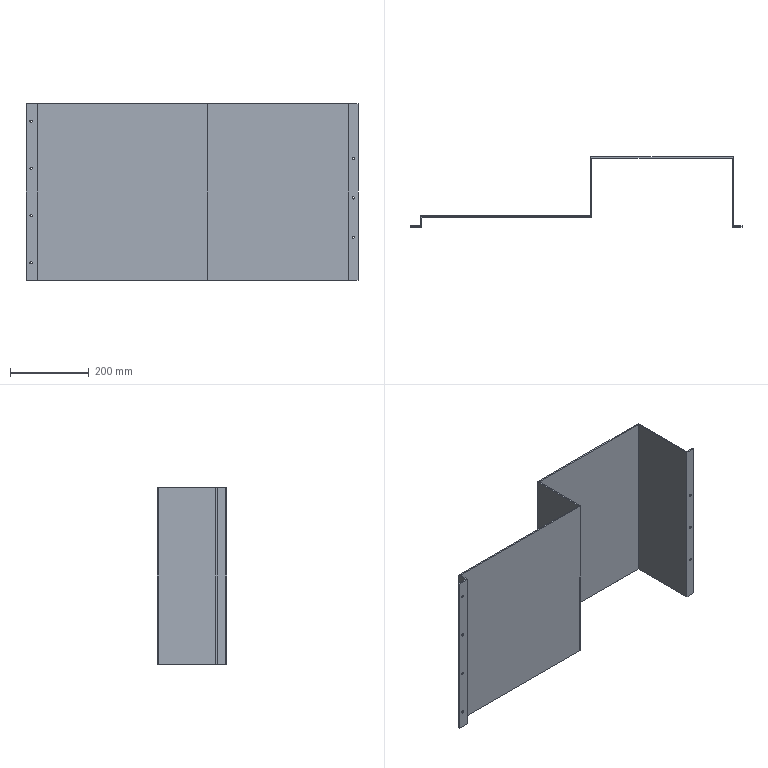Part | STEP file | Guard 4 | 1 solid | 32 faces | box 845 x 178 x 450 mm | volume 1612656 mm3 | plane 18 | cylinder 14 | commonest cylinder face diameters 6 x14
STEP:
#1=CARTESIAN_POINT('',(-415.,-25.,-60.));
#2=VERTEX_POINT('',#1);
#3=CARTESIAN_POINT('',(-409.,-25.,-60.));
#4=VERTEX_POINT('',#3);
#5=CARTESIAN_POINT('',(-412.,-25.,-60.));
#6=DIRECTION('',(0.,-1.,0.));
#7=DIRECTION('',(0.,0.,-1.));
#8=AXIS2_PLACEMENT_3D('',#5,#6,#7);
#9=CIRCLE('',#8,3.);
#10=EDGE_CURVE('',#2,#4,#9,.T.);
#11=ORIENTED_EDGE('',*,*,#10,.T.);
#12=CARTESIAN_POINT('',(-409.,-22.,-60.));
#13=VERTEX_POINT('',#12);
#14=CARTESIAN_POINT('',(-409.,-32.,-60.));
#15=DIRECTION('',(0.,1.,0.));
#16=VECTOR('',#15,1000.);
#17=LINE('',#14,#16);
#18=EDGE_CURVE('',#4,#13,#17,.T.);
#19=ORIENTED_EDGE('',*,*,#18,.T.);
#20=CARTESIAN_POINT('',(-415.,-22.,-60.));
#21=VERTEX_POINT('',#20);
#22=CARTESIAN_POINT('',(-412.,-22.,-60.));
#23=DIRECTION('',(0.,1.,0.));
#24=DIRECTION('',(-1.,0.,0.));
#25=AXIS2_PLACEMENT_3D('',#22,#23,#24);
#26=CIRCLE('',#25,3.);
#27=EDGE_CURVE('',#13,#21,#26,.T.);
#28=ORIENTED_EDGE('',*,*,#27,.T.);
#29=CARTESIAN_POINT('',(-415.,-32.,-60.));
#30=DIRECTION('',(0.,1.,0.));
#31=VECTOR('',#30,1000.);
#32=LINE('',#29,#31);
#33=EDGE_CURVE('',#2,#21,#32,.T.);
#34=ORIENTED_EDGE('',*,*,#33,.F.);
#35=EDGE_LOOP('',(#11,#19,#28,#34));
#36=FACE_OUTER_BOUND('',#35,.T.);
#37=CARTESIAN_POINT('',(-412.,-32.,-60.));
#38=DIRECTION('',(0.,1.,0.));
#39=DIRECTION('',(-1.,0.,0.));
#40=AXIS2_PLACEMENT_3D('',#37,#38,#39);
#41=CYLINDRICAL_SURFACE('',#40,3.);
#42=ADVANCED_FACE('',(#36),#41,.F.);
#43=CARTESIAN_POINT('',(-415.,-25.,60.));
#44=VERTEX_POINT('',#43);
#45=CARTESIAN_POINT('',(-409.,-25.,60.));
#46=VERTEX_POINT('',#45);
#47=CARTESIAN_POINT('',(-412.,-25.,60.));
#48=DIRECTION('',(0.,-1.,0.));
#49=DIRECTION('',(0.,0.,-1.));
#50=AXIS2_PLACEMENT_3D('',#47,#48,#49);
#51=CIRCLE('',#50,3.);
#52=EDGE_CURVE('',#44,#46,#51,.T.);
#53=ORIENTED_EDGE('',*,*,#52,.T.);
#54=CARTESIAN_POINT('',(-409.,-22.,60.));
#55=VERTEX_POINT('',#54);
#56=CARTESIAN_POINT('',(-409.,-32.,60.));
#57=DIRECTION('',(0.,1.,0.));
#58=VECTOR('',#57,1000.);
#59=LINE('',#56,#58);
#60=EDGE_CURVE('',#46,#55,#59,.T.);
#61=ORIENTED_EDGE('',*,*,#60,.T.);
#62=CARTESIAN_POINT('',(-415.,-22.,60.));
#63=VERTEX_POINT('',#62);
#64=CARTESIAN_POINT('',(-412.,-22.,60.));
#65=DIRECTION('',(0.,1.,0.));
#66=DIRECTION('',(-1.,0.,0.));
#67=AXIS2_PLACEMENT_3D('',#64,#65,#66);
#68=CIRCLE('',#67,3.);
#69=EDGE_CURVE('',#55,#63,#68,.T.);
#70=ORIENTED_EDGE('',*,*,#69,.T.);
#71=CARTESIAN_POINT('',(-415.,-32.,60.));
#72=DIRECTION('',(0.,1.,0.));
#73=VECTOR('',#72,1000.);
#74=LINE('',#71,#73);
#75=EDGE_CURVE('',#44,#63,#74,.T.);
#76=ORIENTED_EDGE('',*,*,#75,.F.);
#77=EDGE_LOOP('',(#53,#61,#70,#76));
#78=FACE_OUTER_BOUND('',#77,.T.);
#79=CARTESIAN_POINT('',(-412.,-32.,60.));
#80=DIRECTION('',(0.,1.,0.));
#81=DIRECTION('',(-1.,0.,0.));
#82=AXIS2_PLACEMENT_3D('',#79,#80,#81);
#83=CYLINDRICAL_SURFACE('',#82,3.);
#84=ADVANCED_FACE('',(#78),#83,.F.);
#85=CARTESIAN_POINT('',(-415.,-25.,180.));
#86=VERTEX_POINT('',#85);
#87=CARTESIAN_POINT('',(-409.,-25.,180.));
#88=VERTEX_POINT('',#87);
#89=CARTESIAN_POINT('',(-412.,-25.,180.));
#90=DIRECTION('',(0.,-1.,0.));
#91=DIRECTION('',(0.,0.,-1.));
#92=AXIS2_PLACEMENT_3D('',#89,#90,#91);
#93=CIRCLE('',#92,3.);
#94=EDGE_CURVE('',#86,#88,#93,.T.);
#95=ORIENTED_EDGE('',*,*,#94,.T.);
#96=CARTESIAN_POINT('',(-409.,-22.,180.));
#97=VERTEX_POINT('',#96);
#98=CARTESIAN_POINT('',(-409.,-32.,180.));
#99=DIRECTION('',(0.,1.,0.));
#100=VECTOR('',#99,1000.);
#101=LINE('',#98,#100);
#102=EDGE_CURVE('',#88,#97,#101,.T.);
#103=ORIENTED_EDGE('',*,*,#102,.T.);
#104=CARTESIAN_POINT('',(-415.,-22.,180.));
#105=VERTEX_POINT('',#104);
#106=CARTESIAN_POINT('',(-412.,-22.,180.));
#107=DIRECTION('',(0.,1.,0.));
#108=DIRECTION('',(-1.,0.,0.));
#109=AXIS2_PLACEMENT_3D('',#106,#107,#108);
#110=CIRCLE('',#109,3.);
#111=EDGE_CURVE('',#97,#105,#110,.T.);
#112=ORIENTED_EDGE('',*,*,#111,.T.);
#113=CARTESIAN_POINT('',(-415.,-32.,180.));
#114=DIRECTION('',(0.,1.,0.));
#115=VECTOR('',#114,1000.);
#116=LINE('',#113,#115);
#117=EDGE_CURVE('',#86,#105,#116,.T.);
#118=ORIENTED_EDGE('',*,*,#117,.F.);
#119=EDGE_LOOP('',(#95,#103,#112,#118));
#120=FACE_OUTER_BOUND('',#119,.T.);
#121=CARTESIAN_POINT('',(-412.,-32.,180.));
#122=DIRECTION('',(0.,1.,0.));
#123=DIRECTION('',(-1.,0.,0.));
#124=AXIS2_PLACEMENT_3D('',#121,#122,#123);
#125=CYLINDRICAL_SURFACE('',#124,3.);
#126=ADVANCED_FACE('',(#120),#125,.F.);
#127=CARTESIAN_POINT('',(-415.,-25.,-180.));
#128=VERTEX_POINT('',#127);
#129=CARTESIAN_POINT('',(-409.,-25.,-180.));
#130=VERTEX_POINT('',#129);
#131=CARTESIAN_POINT('',(-412.,-25.,-180.));
#132=DIRECTION('',(0.,-1.,0.));
#133=DIRECTION('',(0.,0.,-1.));
#134=AXIS2_PLACEMENT_3D('',#131,#132,#133);
#135=CIRCLE('',#134,3.);
#136=EDGE_CURVE('',#128,#130,#135,.T.);
#137=ORIENTED_EDGE('',*,*,#136,.T.);
#138=CARTESIAN_POINT('',(-409.,-22.,-180.));
#139=VERTEX_POINT('',#138);
#140=CARTESIAN_POINT('',(-409.,-32.,-180.));
#141=DIRECTION('',(0.,1.,0.));
#142=VECTOR('',#141,1000.);
#143=LINE('',#140,#142);
#144=EDGE_CURVE('',#130,#139,#143,.T.);
#145=ORIENTED_EDGE('',*,*,#144,.T.);
#146=CARTESIAN_POINT('',(-415.,-22.,-180.));
#147=VERTEX_POINT('',#146);
#148=CARTESIAN_POINT('',(-412.,-22.,-180.));
#149=DIRECTION('',(0.,1.,0.));
#150=DIRECTION('',(-1.,0.,0.));
#151=AXIS2_PLACEMENT_3D('',#148,#149,#150);
#152=CIRCLE('',#151,3.);
#153=EDGE_CURVE('',#139,#147,#152,.T.);
#154=ORIENTED_EDGE('',*,*,#153,.T.);
#155=CARTESIAN_POINT('',(-415.,-32.,-180.));
#156=DIRECTION('',(0.,1.,0.));
#157=VECTOR('',#156,1000.);
#158=LINE('',#155,#157);
#159=EDGE_CURVE('',#128,#147,#158,.T.);
#160=ORIENTED_EDGE('',*,*,#159,.F.);
#161=EDGE_LOOP('',(#137,#145,#154,#160));
#162=FACE_OUTER_BOUND('',#161,.T.);
#163=CARTESIAN_POINT('',(-412.,-32.,-180.));
#164=DIRECTION('',(0.,1.,0.));
#165=DIRECTION('',(-1.,0.,0.));
#166=AXIS2_PLACEMENT_3D('',#163,#164,#165);
#167=CYLINDRICAL_SURFACE('',#166,3.);
#168=ADVANCED_FACE('',(#162),#167,.F.);
#169=CARTESIAN_POINT('',(411.,-25.,-115.));
#170=VERTEX_POINT('',#169);
#171=CARTESIAN_POINT('',(405.,-25.,-115.));
#172=VERTEX_POINT('',#171);
#173=CARTESIAN_POINT('',(408.,-25.,-115.));
#174=DIRECTION('',(0.,1.,0.));
#175=DIRECTION('',(0.,0.,1.));
#176=AXIS2_PLACEMENT_3D('',#173,#174,#175);
#177=CIRCLE('',#176,3.);
#178=EDGE_CURVE('',#170,#172,#177,.T.);
#179=ORIENTED_EDGE('',*,*,#178,.F.);
#180=CARTESIAN_POINT('',(411.,-22.,-115.));
#181=VERTEX_POINT('',#180);
#182=CARTESIAN_POINT('',(411.,-472.,-115.));
#183=DIRECTION('',(0.,1.,0.));
#184=VECTOR('',#183,1000.);
#185=LINE('',#182,#184);
#186=EDGE_CURVE('',#170,#181,#185,.T.);
#187=ORIENTED_EDGE('',*,*,#186,.T.);
#188=CARTESIAN_POINT('',(405.,-22.,-115.));
#189=VERTEX_POINT('',#188);
#190=CARTESIAN_POINT('',(408.,-22.,-115.));
#191=DIRECTION('',(0.,1.,0.));
#192=DIRECTION('',(-1.,0.,0.));
#193=AXIS2_PLACEMENT_3D('',#190,#191,#192);
#194=CIRCLE('',#193,3.);
#195=EDGE_CURVE('',#181,#189,#194,.T.);
#196=ORIENTED_EDGE('',*,*,#195,.T.);
#197=CARTESIAN_POINT('',(405.,-472.,-115.));
#198=DIRECTION('',(0.,1.,0.));
#199=VECTOR('',#198,1000.);
#200=LINE('',#197,#199);
#201=EDGE_CURVE('',#172,#189,#200,.T.);
#202=ORIENTED_EDGE('',*,*,#201,.F.);
#203=EDGE_LOOP('',(#179,#187,#196,#202));
#204=FACE_OUTER_BOUND('',#203,.T.);
#205=CARTESIAN_POINT('',(408.,-472.,-115.));
#206=DIRECTION('',(0.,1.,0.));
#207=DIRECTION('',(-1.,0.,0.));
#208=AXIS2_PLACEMENT_3D('',#205,#206,#207);
#209=CYLINDRICAL_SURFACE('',#208,3.);
#210=ADVANCED_FACE('',(#204),#209,.F.);
#211=CARTESIAN_POINT('',(411.,-25.,-15.));
#212=VERTEX_POINT('',#211);
#213=CARTESIAN_POINT('',(405.,-25.,-15.));
#214=VERTEX_POINT('',#213);
#215=CARTESIAN_POINT('',(408.,-25.,-15.));
#216=DIRECTION('',(0.,1.,0.));
#217=DIRECTION('',(0.,0.,1.));
#218=AXIS2_PLACEMENT_3D('',#215,#216,#217);
#219=CIRCLE('',#218,3.);
#220=EDGE_CURVE('',#212,#214,#219,.T.);
#221=ORIENTED_EDGE('',*,*,#220,.F.);
#222=CARTESIAN_POINT('',(411.,-22.,-15.));
#223=VERTEX_POINT('',#222);
#224=CARTESIAN_POINT('',(411.,-472.,-15.));
#225=DIRECTION('',(0.,1.,0.));
#226=VECTOR('',#225,1000.);
#227=LINE('',#224,#226);
#228=EDGE_CURVE('',#212,#223,#227,.T.);
#229=ORIENTED_EDGE('',*,*,#228,.T.);
#230=CARTESIAN_POINT('',(405.,-22.,-15.));
#231=VERTEX_POINT('',#230);
#232=CARTESIAN_POINT('',(408.,-22.,-15.));
#233=DIRECTION('',(0.,1.,0.));
#234=DIRECTION('',(-1.,0.,0.));
#235=AXIS2_PLACEMENT_3D('',#232,#233,#234);
#236=CIRCLE('',#235,3.);
#237=EDGE_CURVE('',#223,#231,#236,.T.);
#238=ORIENTED_EDGE('',*,*,#237,.T.);
#239=CARTESIAN_POINT('',(405.,-472.,-15.));
#240=DIRECTION('',(0.,1.,0.));
#241=VECTOR('',#240,1000.);
#242=LINE('',#239,#241);
#243=EDGE_CURVE('',#214,#231,#242,.T.);
#244=ORIENTED_EDGE('',*,*,#243,.F.);
#245=EDGE_LOOP('',(#221,#229,#238,#244));
#246=FACE_OUTER_BOUND('',#245,.T.);
#247=CARTESIAN_POINT('',(408.,-472.,-15.));
#248=DIRECTION('',(0.,1.,0.));
#249=DIRECTION('',(-1.,0.,0.));
#250=AXIS2_PLACEMENT_3D('',#247,#248,#249);
#251=CYLINDRICAL_SURFACE('',#250,3.);
#252=ADVANCED_FACE('',(#246),#251,.F.);
#253=CARTESIAN_POINT('',(411.,-25.,85.));
#254=VERTEX_POINT('',#253);
#255=CARTESIAN_POINT('',(405.,-25.,85.));
#256=VERTEX_POINT('',#255);
#257=CARTESIAN_POINT('',(408.,-25.,85.));
#258=DIRECTION('',(0.,1.,0.));
#259=DIRECTION('',(0.,0.,1.));
#260=AXIS2_PLACEMENT_3D('',#257,#258,#259);
#261=CIRCLE('',#260,3.);
#262=EDGE_CURVE('',#254,#256,#261,.T.);
#263=ORIENTED_EDGE('',*,*,#262,.F.);
#264=CARTESIAN_POINT('',(411.,-22.,85.));
#265=VERTEX_POINT('',#264);
#266=CARTESIAN_POINT('',(411.,-472.,85.));
#267=DIRECTION('',(0.,1.,0.));
#268=VECTOR('',#267,1000.);
#269=LINE('',#266,#268);
#270=EDGE_CURVE('',#254,#265,#269,.T.);
#271=ORIENTED_EDGE('',*,*,#270,.T.);
#272=CARTESIAN_POINT('',(405.,-22.,85.));
#273=VERTEX_POINT('',#272);
#274=CARTESIAN_POINT('',(408.,-22.,85.));
#275=DIRECTION('',(0.,1.,0.));
#276=DIRECTION('',(-1.,0.,0.));
#277=AXIS2_PLACEMENT_3D('',#274,#275,#276);
#278=CIRCLE('',#277,3.);
#279=EDGE_CURVE('',#265,#273,#278,.T.);
#280=ORIENTED_EDGE('',*,*,#279,.T.);
#281=CARTESIAN_POINT('',(405.,-472.,85.));
#282=DIRECTION('',(0.,1.,0.));
#283=VECTOR('',#282,1000.);
#284=LINE('',#281,#283);
#285=EDGE_CURVE('',#256,#273,#284,.T.);
#286=ORIENTED_EDGE('',*,*,#285,.F.);
#287=EDGE_LOOP('',(#263,#271,#280,#286));
#288=FACE_OUTER_BOUND('',#287,.T.);
#289=CARTESIAN_POINT('',(408.,-472.,85.));
#290=DIRECTION('',(0.,1.,0.));
#291=DIRECTION('',(-1.,0.,0.));
#292=AXIS2_PLACEMENT_3D('',#289,#290,#291);
#293=CYLINDRICAL_SURFACE('',#292,3.);
#294=ADVANCED_FACE('',(#288),#293,.F.);
#295=CARTESIAN_POINT('',(395.,-25.,-225.));
#296=VERTEX_POINT('',#295);
#297=CARTESIAN_POINT('',(395.,150.,-225.));
#298=VERTEX_POINT('',#297);
#299=CARTESIAN_POINT('',(395.,0.,-225.));
#300=DIRECTION('',(0.,1.,0.));
#301=VECTOR('',#300,1000.);
#302=LINE('',#299,#301);
#303=EDGE_CURVE('',#296,#298,#302,.T.);
#304=ORIENTED_EDGE('',*,*,#303,.F.);
#305=CARTESIAN_POINT('',(395.,-25.,225.));
#306=VERTEX_POINT('',#305);
#307=CARTESIAN_POINT('',(395.,-25.,225.));
#308=DIRECTION('',(0.,0.,-1.));
#309=VECTOR('',#308,1000.);
#310=LINE('',#307,#309);
#311=EDGE_CURVE('',#306,#296,#310,.T.);
#312=ORIENTED_EDGE('',*,*,#311,.F.);
#313=CARTESIAN_POINT('',(395.,150.,225.));
#314=VERTEX_POINT('',#313);
#315=CARTESIAN_POINT('',(395.,0.,225.));
#316=DIRECTION('',(0.,1.,0.));
#317=VECTOR('',#316,1000.);
#318=LINE('',#315,#317);
#319=EDGE_CURVE('',#306,#314,#318,.T.);
#320=ORIENTED_EDGE('',*,*,#319,.T.);
#321=CARTESIAN_POINT('',(395.,150.,225.));
#322=DIRECTION('',(0.,0.,-1.));
#323=VECTOR('',#322,1000.);
#324=LINE('',#321,#323);
#325=EDGE_CURVE('',#314,#298,#324,.T.);
#326=ORIENTED_EDGE('',*,*,#325,.T.);
#327=EDGE_LOOP('',(#304,#312,#320,#326));
#328=FACE_OUTER_BOUND('',#327,.T.);
#329=CARTESIAN_POINT('',(395.,0.,225.));
#330=DIRECTION('',(-1.,0.,0.));
#331=DIRECTION('',(0.,0.,1.));
#332=AXIS2_PLACEMENT_3D('',#329,#330,#331);
#333=PLANE('',#332);
#334=ADVANCED_FACE('',(#328),#333,.T.);
#335=CARTESIAN_POINT('',(408.,-25.,-115.));
#336=DIRECTION('',(0.,1.,0.));
#337=DIRECTION('',(0.,0.,1.));
#338=AXIS2_PLACEMENT_3D('',#335,#336,#337);
#339=CIRCLE('',#338,3.);
#340=EDGE_CURVE('',#172,#170,#339,.T.);
#341=ORIENTED_EDGE('',*,*,#340,.T.);
#342=ORIENTED_EDGE('',*,*,#178,.T.);
#343=EDGE_LOOP('',(#341,#342));
#344=FACE_BOUND('',#343,.T.);
#345=CARTESIAN_POINT('',(408.,-25.,-15.));
#346=DIRECTION('',(0.,1.,0.));
#347=DIRECTION('',(0.,0.,1.));
#348=AXIS2_PLACEMENT_3D('',#345,#346,#347);
#349=CIRCLE('',#348,3.);
#350=EDGE_CURVE('',#214,#212,#349,.T.);
#351=ORIENTED_EDGE('',*,*,#350,.T.);
#352=ORIENTED_EDGE('',*,*,#220,.T.);
#353=EDGE_LOOP('',(#351,#352));
#354=FACE_BOUND('',#353,.T.);
#355=CARTESIAN_POINT('',(408.,-25.,85.));
#356=DIRECTION('',(0.,1.,0.));
#357=DIRECTION('',(0.,0.,1.));
#358=AXIS2_PLACEMENT_3D('',#355,#356,#357);
#359=CIRCLE('',#358,3.);
#360=EDGE_CURVE('',#256,#254,#359,.T.);
#361=ORIENTED_EDGE('',*,*,#360,.T.);
#362=ORIENTED_EDGE('',*,*,#262,.T.);
#363=EDGE_LOOP('',(#361,#362));
#364=FACE_BOUND('',#363,.T.);
#365=CARTESIAN_POINT('',(420.,-25.,-225.));
#366=VERTEX_POINT('',#365);
#367=CARTESIAN_POINT('',(0.,-25.,-225.));
#368=DIRECTION('',(1.,0.,0.));
#369=VECTOR('',#368,1000.);
#370=LINE('',#367,#369);
#371=EDGE_CURVE('',#296,#366,#370,.T.);
#372=ORIENTED_EDGE('',*,*,#371,.T.);
#373=CARTESIAN_POINT('',(420.,-25.,225.));
#374=VERTEX_POINT('',#373);
#375=CARTESIAN_POINT('',(420.,-25.,225.));
#376=DIRECTION('',(0.,0.,1.));
#377=VECTOR('',#376,1000.);
#378=LINE('',#375,#377);
#379=EDGE_CURVE('',#366,#374,#378,.T.);
#380=ORIENTED_EDGE('',*,*,#379,.T.);
#381=CARTESIAN_POINT('',(0.,-25.,225.));
#382=DIRECTION('',(1.,0.,0.));
#383=VECTOR('',#382,1000.);
#384=LINE('',#381,#383);
#385=EDGE_CURVE('',#306,#374,#384,.T.);
#386=ORIENTED_EDGE('',*,*,#385,.F.);
#387=ORIENTED_EDGE('',*,*,#311,.T.);
#388=EDGE_LOOP('',(#372,#380,#386,#387));
#389=FACE_OUTER_BOUND('',#388,.T.);
#390=CARTESIAN_POINT('',(0.,-25.,225.));
#391=DIRECTION('',(0.,1.,0.));
#392=DIRECTION('',(0.,0.,1.));
#393=AXIS2_PLACEMENT_3D('',#390,#391,#392);
#394=PLANE('',#393);
#395=ADVANCED_FACE('',(#344,#354,#364,#389),#394,.F.);
#396=CARTESIAN_POINT('',(408.,-22.,-115.));
#397=DIRECTION('',(0.,1.,0.));
#398=DIRECTION('',(-1.,0.,0.));
#399=AXIS2_PLACEMENT_3D('',#396,#397,#398);
#400=CIRCLE('',#399,3.);
#401=EDGE_CURVE('',#189,#181,#400,.T.);
#402=ORIENTED_EDGE('',*,*,#401,.F.);
#403=ORIENTED_EDGE('',*,*,#195,.F.);
#404=EDGE_LOOP('',(#402,#403));
#405=FACE_BOUND('',#404,.T.);
#406=CARTESIAN_POINT('',(408.,-22.,-15.));
#407=DIRECTION('',(0.,1.,0.));
#408=DIRECTION('',(-1.,0.,0.));
#409=AXIS2_PLACEMENT_3D('',#406,#407,#408);
#410=CIRCLE('',#409,3.);
#411=EDGE_CURVE('',#231,#223,#410,.T.);
#412=ORIENTED_EDGE('',*,*,#411,.F.);
#413=ORIENTED_EDGE('',*,*,#237,.F.);
#414=EDGE_LOOP('',(#412,#413));
#415=FACE_BOUND('',#414,.T.);
#416=CARTESIAN_POINT('',(408.,-22.,85.));
#417=DIRECTION('',(0.,1.,0.));
#418=DIRECTION('',(-1.,0.,0.));
#419=AXIS2_PLACEMENT_3D('',#416,#417,#418);
#420=CIRCLE('',#419,3.);
#421=EDGE_CURVE('',#273,#265,#420,.T.);
#422=ORIENTED_EDGE('',*,*,#421,.F.);
#423=ORIENTED_EDGE('',*,*,#279,.F.);
#424=EDGE_LOOP('',(#422,#423));
#425=FACE_BOUND('',#424,.T.);
#426=CARTESIAN_POINT('',(420.,-22.,-225.));
#427=VERTEX_POINT('',#426);
#428=CARTESIAN_POINT('',(420.,-22.,225.));
#429=VERTEX_POINT('',#428);
#430=CARTESIAN_POINT('',(420.,-22.,225.));
#431=DIRECTION('',(0.,0.,1.));
#432=VECTOR('',#431,1000.);
#433=LINE('',#430,#432);
#434=EDGE_CURVE('',#427,#429,#433,.T.);
#435=ORIENTED_EDGE('',*,*,#434,.F.);
#436=CARTESIAN_POINT('',(398.,-22.,-225.));
#437=VERTEX_POINT('',#436);
#438=CARTESIAN_POINT('',(0.,-22.,-225.));
#439=DIRECTION('',(1.,0.,0.));
#440=VECTOR('',#439,1000.);
#441=LINE('',#438,#440);
#442=EDGE_CURVE('',#437,#427,#441,.T.);
#443=ORIENTED_EDGE('',*,*,#442,.F.);
#444=CARTESIAN_POINT('',(398.,-22.,225.));
#445=VERTEX_POINT('',#444);
#446=CARTESIAN_POINT('',(398.,-22.,225.));
#447=DIRECTION('',(0.,0.,-1.));
#448=VECTOR('',#447,1000.);
#449=LINE('',#446,#448);
#450=EDGE_CURVE('',#445,#437,#449,.T.);
#451=ORIENTED_EDGE('',*,*,#450,.F.);
#452=CARTESIAN_POINT('',(0.,-22.,225.));
#453=DIRECTION('',(1.,0.,0.));
#454=VECTOR('',#453,1000.);
#455=LINE('',#452,#454);
#456=EDGE_CURVE('',#445,#429,#455,.T.);
#457=ORIENTED_EDGE('',*,*,#456,.T.);
#458=EDGE_LOOP('',(#435,#443,#451,#457));
#459=FACE_OUTER_BOUND('',#458,.T.);
#460=CARTESIAN_POINT('',(0.,-22.,225.));
#461=DIRECTION('',(0.,1.,0.));
#462=DIRECTION('',(-1.,0.,0.));
#463=AXIS2_PLACEMENT_3D('',#460,#461,#462);
#464=PLANE('',#463);
#465=ADVANCED_FACE('',(#405,#415,#425,#459),#464,.T.);
#466=CARTESIAN_POINT('',(398.,153.,-225.));
#467=VERTEX_POINT('',#466);
#468=CARTESIAN_POINT('',(398.,0.,-225.));
#469=DIRECTION('',(0.,-1.,0.));
#470=VECTOR('',#469,1000.);
#471=LINE('',#468,#470);
#472=EDGE_CURVE('',#467,#437,#471,.T.);
#473=ORIENTED_EDGE('',*,*,#472,.F.);
#474=CARTESIAN_POINT('',(398.,153.,225.));
#475=VERTEX_POINT('',#474);
#476=CARTESIAN_POINT('',(398.,153.,225.));
#477=DIRECTION('',(0.,0.,-1.));
#478=VECTOR('',#477,1000.);
#479=LINE('',#476,#478);
#480=EDGE_CURVE('',#475,#467,#479,.T.);
#481=ORIENTED_EDGE('',*,*,#480,.F.);
#482=CARTESIAN_POINT('',(398.,0.,225.));
#483=DIRECTION('',(0.,-1.,0.));
#484=VECTOR('',#483,1000.);
#485=LINE('',#482,#484);
#486=EDGE_CURVE('',#475,#445,#485,.T.);
#487=ORIENTED_EDGE('',*,*,#486,.T.);
#488=ORIENTED_EDGE('',*,*,#450,.T.);
#489=EDGE_LOOP('',(#473,#481,#487,#488));
#490=FACE_OUTER_BOUND('',#489,.T.);
#491=CARTESIAN_POINT('',(398.,0.,225.));
#492=DIRECTION('',(1.,0.,0.));
#493=DIRECTION('',(0.,0.,-1.));
#494=AXIS2_PLACEMENT_3D('',#491,#492,#493);
#495=PLANE('',#494);
#496=ADVANCED_FACE('',(#490),#495,.T.);
#497=CARTESIAN_POINT('',(35.,153.,-225.));
#498=VERTEX_POINT('',#497);
#499=CARTESIAN_POINT('',(0.,153.,-225.));
#500=DIRECTION('',(-1.,0.,0.));
#501=VECTOR('',#500,1000.);
#502=LINE('',#499,#501);
#503=EDGE_CURVE('',#467,#498,#502,.T.);
#504=ORIENTED_EDGE('',*,*,#503,.T.);
#505=CARTESIAN_POINT('',(35.,153.,225.));
#506=VERTEX_POINT('',#505);
#507=CARTESIAN_POINT('',(35.,153.,225.));
#508=DIRECTION('',(0.,0.,-1.));
#509=VECTOR('',#508,1000.);
#510=LINE('',#507,#509);
#511=EDGE_CURVE('',#506,#498,#510,.T.);
#512=ORIENTED_EDGE('',*,*,#511,.F.);
#513=CARTESIAN_POINT('',(0.,153.,225.));
#514=DIRECTION('',(-1.,0.,0.));
#515=VECTOR('',#514,1000.);
#516=LINE('',#513,#515);
#517=EDGE_CURVE('',#475,#506,#516,.T.);
#518=ORIENTED_EDGE('',*,*,#517,.F.);
#519=ORIENTED_EDGE('',*,*,#480,.T.);
#520=EDGE_LOOP('',(#504,#512,#518,#519));
#521=FACE_OUTER_BOUND('',#520,.T.);
#522=CARTESIAN_POINT('',(0.,153.,225.));
#523=DIRECTION('',(0.,-1.,0.));
#524=DIRECTION('',(1.,0.,0.));
#525=AXIS2_PLACEMENT_3D('',#522,#523,#524);
#526=PLANE('',#525);
#527=ADVANCED_FACE('',(#521),#526,.F.);
#528=CARTESIAN_POINT('',(35.,3.,-225.));
#529=VERTEX_POINT('',#528);
#530=CARTESIAN_POINT('',(35.,0.,-225.));
#531=DIRECTION('',(0.,-1.,0.));
#532=VECTOR('',#531,1000.);
#533=LINE('',#530,#532);
#534=EDGE_CURVE('',#498,#529,#533,.T.);
#535=ORIENTED_EDGE('',*,*,#534,.T.);
#536=CARTESIAN_POINT('',(35.,3.,225.));
#537=VERTEX_POINT('',#536);
#538=CARTESIAN_POINT('',(35.,3.,225.));
#539=DIRECTION('',(0.,0.,-1.));
#540=VECTOR('',#539,1000.);
#541=LINE('',#538,#540);
#542=EDGE_CURVE('',#537,#529,#541,.T.);
#543=ORIENTED_EDGE('',*,*,#542,.F.);
#544=CARTESIAN_POINT('',(35.,0.,225.));
#545=DIRECTION('',(0.,-1.,0.));
#546=VECTOR('',#545,1000.);
#547=LINE('',#544,#546);
#548=EDGE_CURVE('',#506,#537,#547,.T.);
#549=ORIENTED_EDGE('',*,*,#548,.F.);
#550=ORIENTED_EDGE('',*,*,#511,.T.);
#551=EDGE_LOOP('',(#535,#543,#549,#550));
#552=FACE_OUTER_BOUND('',#551,.T.);
#553=CARTESIAN_POINT('',(35.,0.,225.));
#554=DIRECTION('',(1.,0.,0.));
#555=DIRECTION('',(0.,1.,0.));
#556=AXIS2_PLACEMENT_3D('',#553,#554,#555);
#557=PLANE('',#556);
#558=ADVANCED_FACE('',(#552),#557,.F.);
#559=CARTESIAN_POINT('',(-398.,3.,-225.));
#560=VERTEX_POINT('',#559);
#561=CARTESIAN_POINT('',(0.,3.,-225.));
#562=DIRECTION('',(1.,0.,0.));
#563=VECTOR('',#562,1000.);
#564=LINE('',#561,#563);
#565=EDGE_CURVE('',#560,#529,#564,.T.);
#566=ORIENTED_EDGE('',*,*,#565,.F.);
#567=CARTESIAN_POINT('',(-398.,3.,225.));
#568=VERTEX_POINT('',#567);
#569=CARTESIAN_POINT('',(-398.,3.,225.));
#570=DIRECTION('',(0.,0.,-1.));
#571=VECTOR('',#570,1000.);
#572=LINE('',#569,#571);
#573=EDGE_CURVE('',#568,#560,#572,.T.);
#574=ORIENTED_EDGE('',*,*,#573,.F.);
#575=CARTESIAN_POINT('',(0.,3.,225.));
#576=DIRECTION('',(1.,0.,0.));
#577=VECTOR('',#576,1000.);
#578=LINE('',#575,#577);
#579=EDGE_CURVE('',#568,#537,#578,.T.);
#580=ORIENTED_EDGE('',*,*,#579,.T.);
#581=ORIENTED_EDGE('',*,*,#542,.T.);
#582=EDGE_LOOP('',(#566,#574,#580,#581));
#583=FACE_OUTER_BOUND('',#582,.T.);
#584=CARTESIAN_POINT('',(0.,3.,225.));
#585=DIRECTION('',(0.,1.,0.));
#586=DIRECTION('',(-1.,0.,0.));
#587=AXIS2_PLACEMENT_3D('',#584,#585,#586);
#588=PLANE('',#587);
#589=ADVANCED_FACE('',(#583),#588,.T.);
#590=CARTESIAN_POINT('',(-398.,-22.,-225.));
#591=VERTEX_POINT('',#590);
#592=CARTESIAN_POINT('',(-398.,0.,-225.));
#593=DIRECTION('',(0.,-1.,0.));
#594=VECTOR('',#593,1000.);
#595=LINE('',#592,#594);
#596=EDGE_CURVE('',#560,#591,#595,.T.);
#597=ORIENTED_EDGE('',*,*,#596,.T.);
#598=CARTESIAN_POINT('',(-398.,-22.,225.));
#599=VERTEX_POINT('',#598);
#600=CARTESIAN_POINT('',(-398.,-22.,225.));
#601=DIRECTION('',(0.,0.,-1.));
#602=VECTOR('',#601,1000.);
#603=LINE('',#600,#602);
#604=EDGE_CURVE('',#599,#591,#603,.T.);
#605=ORIENTED_EDGE('',*,*,#604,.F.);
#606=CARTESIAN_POINT('',(-398.,0.,225.));
#607=DIRECTION('',(0.,-1.,0.));
#608=VECTOR('',#607,1000.);
#609=LINE('',#606,#608);
#610=EDGE_CURVE('',#568,#599,#609,.T.);
#611=ORIENTED_EDGE('',*,*,#610,.F.);
#612=ORIENTED_EDGE('',*,*,#573,.T.);
#613=EDGE_LOOP('',(#597,#605,#611,#612));
#614=FACE_OUTER_BOUND('',#613,.T.);
#615=CARTESIAN_POINT('',(-398.,0.,225.));
#616=DIRECTION('',(1.,0.,0.));
#617=DIRECTION('',(0.,0.,-1.));
#618=AXIS2_PLACEMENT_3D('',#615,#616,#617);
#619=PLANE('',#618);
#620=ADVANCED_FACE('',(#614),#619,.F.);
#621=CARTESIAN_POINT('',(-412.,-22.,-60.));
#622=DIRECTION('',(0.,1.,0.));
#623=DIRECTION('',(-1.,0.,0.));
#624=AXIS2_PLACEMENT_3D('',#621,#622,#623);
#625=CIRCLE('',#624,3.);
#626=EDGE_CURVE('',#21,#13,#625,.T.);
#627=ORIENTED_EDGE('',*,*,#626,.F.);
#628=ORIENTED_EDGE('',*,*,#27,.F.);
#629=EDGE_LOOP('',(#627,#628));
#630=FACE_BOUND('',#629,.T.);
#631=CARTESIAN_POINT('',(-412.,-22.,60.));
#632=DIRECTION('',(0.,1.,0.));
#633=DIRECTION('',(-1.,0.,0.));
#634=AXIS2_PLACEMENT_3D('',#631,#632,#633);
#635=CIRCLE('',#634,3.);
#636=EDGE_CURVE('',#63,#55,#635,.T.);
#637=ORIENTED_EDGE('',*,*,#636,.F.);
#638=ORIENTED_EDGE('',*,*,#69,.F.);
#639=EDGE_LOOP('',(#637,#638));
#640=FACE_BOUND('',#639,.T.);
#641=CARTESIAN_POINT('',(-412.,-22.,180.));
#642=DIRECTION('',(0.,1.,0.));
#643=DIRECTION('',(-1.,0.,0.));
#644=AXIS2_PLACEMENT_3D('',#641,#642,#643);
#645=CIRCLE('',#644,3.);
#646=EDGE_CURVE('',#105,#97,#645,.T.);
#647=ORIENTED_EDGE('',*,*,#646,.F.);
#648=ORIENTED_EDGE('',*,*,#111,.F.);
#649=EDGE_LOOP('',(#647,#648));
#650=FACE_BOUND('',#649,.T.);
#651=CARTESIAN_POINT('',(-412.,-22.,-180.));
#652=DIRECTION('',(0.,1.,0.));
#653=DIRECTION('',(-1.,0.,0.));
#654=AXIS2_PLACEMENT_3D('',#651,#652,#653);
#655=CIRCLE('',#654,3.);
#656=EDGE_CURVE('',#147,#139,#655,.T.);
#657=ORIENTED_EDGE('',*,*,#656,.F.);
#658=ORIENTED_EDGE('',*,*,#153,.F.);
#659=EDGE_LOOP('',(#657,#658));
#660=FACE_BOUND('',#659,.T.);
#661=CARTESIAN_POINT('',(-425.,-22.,-225.));
#662=VERTEX_POINT('',#661);
#663=CARTESIAN_POINT('',(0.,-22.,-225.));
#664=DIRECTION('',(-1.,0.,0.));
#665=VECTOR('',#664,1000.);
#666=LINE('',#663,#665);
#667=EDGE_CURVE('',#591,#662,#666,.T.);
#668=ORIENTED_EDGE('',*,*,#667,.T.);
#669=CARTESIAN_POINT('',(-425.,-22.,225.));
#670=VERTEX_POINT('',#669);
#671=CARTESIAN_POINT('',(-425.,-22.,225.));
#672=DIRECTION('',(0.,0.,-1.));
#673=VECTOR('',#672,1000.);
#674=LINE('',#671,#673);
#675=EDGE_CURVE('',#670,#662,#674,.T.);
#676=ORIENTED_EDGE('',*,*,#675,.F.);
#677=CARTESIAN_POINT('',(0.,-22.,225.));
#678=DIRECTION('',(-1.,0.,0.));
#679=VECTOR('',#678,1000.);
#680=LINE('',#677,#679);
#681=EDGE_CURVE('',#599,#670,#680,.T.);
#682=ORIENTED_EDGE('',*,*,#681,.F.);
#683=ORIENTED_EDGE('',*,*,#604,.T.);
#684=EDGE_LOOP('',(#668,#676,#682,#683));
#685=FACE_OUTER_BOUND('',#684,.T.);
#686=CARTESIAN_POINT('',(0.,-22.,225.));
#687=DIRECTION('',(0.,-1.,0.));
#688=DIRECTION('',(1.,0.,0.));
#689=AXIS2_PLACEMENT_3D('',#686,#687,#688);
#690=PLANE('',#689);
#691=ADVANCED_FACE('',(#630,#640,#650,#660,#685),#690,.F.);
#692=CARTESIAN_POINT('',(-425.,-25.,-225.));
#693=VERTEX_POINT('',#692);
#694=CARTESIAN_POINT('',(-425.,0.,-225.));
#695=DIRECTION('',(0.,1.,0.));
#696=VECTOR('',#695,1000.);
#697=LINE('',#694,#696);
#698=EDGE_CURVE('',#693,#662,#697,.T.);
#699=ORIENTED_EDGE('',*,*,#698,.F.);
#700=CARTESIAN_POINT('',(-425.,-25.,225.));
#701=VERTEX_POINT('',#700);
#702=CARTESIAN_POINT('',(-425.,-25.,225.));
#703=DIRECTION('',(0.,0.,-1.));
#704=VECTOR('',#703,1000.);
#705=LINE('',#702,#704);
#706=EDGE_CURVE('',#701,#693,#705,.T.);
#707=ORIENTED_EDGE('',*,*,#706,.F.);
#708=CARTESIAN_POINT('',(-425.,0.,225.));
#709=DIRECTION('',(0.,1.,0.));
#710=VECTOR('',#709,1000.);
#711=LINE('',#708,#710);
#712=EDGE_CURVE('',#701,#670,#711,.T.);
#713=ORIENTED_EDGE('',*,*,#712,.T.);
#714=ORIENTED_EDGE('',*,*,#675,.T.);
#715=EDGE_LOOP('',(#699,#707,#713,#714));
#716=FACE_OUTER_BOUND('',#715,.T.);
#717=CARTESIAN_POINT('',(-425.,0.,225.));
#718=DIRECTION('',(-1.,0.,0.));
#719=DIRECTION('',(0.,0.,1.));
#720=AXIS2_PLACEMENT_3D('',#717,#718,#719);
#721=PLANE('',#720);
#722=ADVANCED_FACE('',(#716),#721,.T.);
#723=ORIENTED_EDGE('',*,*,#10,.F.);
#724=CARTESIAN_POINT('',(-412.,-25.,-60.));
#725=DIRECTION('',(0.,-1.,0.));
#726=DIRECTION('',(0.,0.,-1.));
#727=AXIS2_PLACEMENT_3D('',#724,#725,#726);
#728=CIRCLE('',#727,3.);
#729=EDGE_CURVE('',#4,#2,#728,.T.);
#730=ORIENTED_EDGE('',*,*,#729,.F.);
#731=EDGE_LOOP('',(#723,#730));
#732=FACE_BOUND('',#731,.T.);
#733=ORIENTED_EDGE('',*,*,#52,.F.);
#734=CARTESIAN_POINT('',(-412.,-25.,60.));
#735=DIRECTION('',(0.,-1.,0.));
#736=DIRECTION('',(0.,0.,-1.));
#737=AXIS2_PLACEMENT_3D('',#734,#735,#736);
#738=CIRCLE('',#737,3.);
#739=EDGE_CURVE('',#46,#44,#738,.T.);
#740=ORIENTED_EDGE('',*,*,#739,.F.);
#741=EDGE_LOOP('',(#733,#740));
#742=FACE_BOUND('',#741,.T.);
#743=ORIENTED_EDGE('',*,*,#94,.F.);
#744=CARTESIAN_POINT('',(-412.,-25.,180.));
#745=DIRECTION('',(0.,-1.,0.));
#746=DIRECTION('',(0.,0.,-1.));
#747=AXIS2_PLACEMENT_3D('',#744,#745,#746);
#748=CIRCLE('',#747,3.);
#749=EDGE_CURVE('',#88,#86,#748,.T.);
#750=ORIENTED_EDGE('',*,*,#749,.F.);
#751=EDGE_LOOP('',(#743,#750));
#752=FACE_BOUND('',#751,.T.);
#753=ORIENTED_EDGE('',*,*,#136,.F.);
#754=CARTESIAN_POINT('',(-412.,-25.,-180.));
#755=DIRECTION('',(0.,-1.,0.));
#756=DIRECTION('',(0.,0.,-1.));
#757=AXIS2_PLACEMENT_3D('',#754,#755,#756);
#758=CIRCLE('',#757,3.);
#759=EDGE_CURVE('',#130,#128,#758,.T.);
#760=ORIENTED_EDGE('',*,*,#759,.F.);
#761=EDGE_LOOP('',(#753,#760));
#762=FACE_BOUND('',#761,.T.);
#763=CARTESIAN_POINT('',(-395.,-25.,-225.));
#764=VERTEX_POINT('',#763);
#765=CARTESIAN_POINT('',(0.,-25.,-225.));
#766=DIRECTION('',(-1.,0.,0.));
#767=VECTOR('',#766,1000.);
#768=LINE('',#765,#767);
#769=EDGE_CURVE('',#764,#693,#768,.T.);
#770=ORIENTED_EDGE('',*,*,#769,.F.);
#771=CARTESIAN_POINT('',(-395.,-25.,225.));
#772=VERTEX_POINT('',#771);
#773=CARTESIAN_POINT('',(-395.,-25.,225.));
#774=DIRECTION('',(0.,0.,-1.));
#775=VECTOR('',#774,1000.);
#776=LINE('',#773,#775);
#777=EDGE_CURVE('',#772,#764,#776,.T.);
#778=ORIENTED_EDGE('',*,*,#777,.F.);
#779=CARTESIAN_POINT('',(0.,-25.,225.));
#780=DIRECTION('',(-1.,0.,0.));
#781=VECTOR('',#780,1000.);
#782=LINE('',#779,#781);
#783=EDGE_CURVE('',#772,#701,#782,.T.);
#784=ORIENTED_EDGE('',*,*,#783,.T.);
#785=ORIENTED_EDGE('',*,*,#706,.T.);
#786=EDGE_LOOP('',(#770,#778,#784,#785));
#787=FACE_OUTER_BOUND('',#786,.T.);
#788=CARTESIAN_POINT('',(0.,-25.,225.));
#789=DIRECTION('',(0.,-1.,0.));
#790=DIRECTION('',(0.,0.,-1.));
#791=AXIS2_PLACEMENT_3D('',#788,#789,#790);
#792=PLANE('',#791);
#793=ADVANCED_FACE('',(#732,#742,#752,#762,#787),#792,.T.);
#794=CARTESIAN_POINT('',(-395.,0.,-225.));
#795=VERTEX_POINT('',#794);
#796=CARTESIAN_POINT('',(-395.,0.,-225.));
#797=DIRECTION('',(0.,-1.,0.));
#798=VECTOR('',#797,1000.);
#799=LINE('',#796,#798);
#800=EDGE_CURVE('',#795,#764,#799,.T.);
#801=ORIENTED_EDGE('',*,*,#800,.F.);
#802=CARTESIAN_POINT('',(-395.,0.,225.));
#803=VERTEX_POINT('',#802);
#804=CARTESIAN_POINT('',(-395.,0.,225.));
#805=DIRECTION('',(0.,0.,-1.));
#806=VECTOR('',#805,1000.);
#807=LINE('',#804,#806);
#808=EDGE_CURVE('',#803,#795,#807,.T.);
#809=ORIENTED_EDGE('',*,*,#808,.F.);
#810=CARTESIAN_POINT('',(-395.,0.,225.));
#811=DIRECTION('',(0.,-1.,0.));
#812=VECTOR('',#811,1000.);
#813=LINE('',#810,#812);
#814=EDGE_CURVE('',#803,#772,#813,.T.);
#815=ORIENTED_EDGE('',*,*,#814,.T.);
#816=ORIENTED_EDGE('',*,*,#777,.T.);
#817=EDGE_LOOP('',(#801,#809,#815,#816));
#818=FACE_OUTER_BOUND('',#817,.T.);
#819=CARTESIAN_POINT('',(-395.,0.,225.));
#820=DIRECTION('',(1.,0.,0.));
#821=DIRECTION('',(0.,0.,-1.));
#822=AXIS2_PLACEMENT_3D('',#819,#820,#821);
#823=PLANE('',#822);
#824=ADVANCED_FACE('',(#818),#823,.T.);
#825=CARTESIAN_POINT('',(38.,0.,-225.));
#826=VERTEX_POINT('',#825);
#827=CARTESIAN_POINT('',(0.,0.,-225.));
#828=DIRECTION('',(-1.,0.,0.));
#829=VECTOR('',#828,1000.);
#830=LINE('',#827,#829);
#831=EDGE_CURVE('',#826,#795,#830,.T.);
#832=ORIENTED_EDGE('',*,*,#831,.F.);
#833=CARTESIAN_POINT('',(38.,0.,225.));
#834=VERTEX_POINT('',#833);
#835=CARTESIAN_POINT('',(38.,0.,225.));
#836=DIRECTION('',(0.,0.,-1.));
#837=VECTOR('',#836,1000.);
#838=LINE('',#835,#837);
#839=EDGE_CURVE('',#834,#826,#838,.T.);
#840=ORIENTED_EDGE('',*,*,#839,.F.);
#841=CARTESIAN_POINT('',(0.,0.,225.));
#842=DIRECTION('',(-1.,0.,0.));
#843=VECTOR('',#842,1000.);
#844=LINE('',#841,#843);
#845=EDGE_CURVE('',#834,#803,#844,.T.);
#846=ORIENTED_EDGE('',*,*,#845,.T.);
#847=ORIENTED_EDGE('',*,*,#808,.T.);
#848=EDGE_LOOP('',(#832,#840,#846,#847));
#849=FACE_OUTER_BOUND('',#848,.T.);
#850=CARTESIAN_POINT('',(0.,0.,225.));
#851=DIRECTION('',(0.,-1.,0.));
#852=DIRECTION('',(1.,0.,0.));
#853=AXIS2_PLACEMENT_3D('',#850,#851,#852);
#854=PLANE('',#853);
#855=ADVANCED_FACE('',(#849),#854,.T.);
#856=CARTESIAN_POINT('',(38.,150.,-225.));
#857=VERTEX_POINT('',#856);
#858=CARTESIAN_POINT('',(38.,0.,-225.));
#859=DIRECTION('',(0.,-1.,0.));
#860=VECTOR('',#859,1000.);
#861=LINE('',#858,#860);
#862=EDGE_CURVE('',#857,#826,#861,.T.);
#863=ORIENTED_EDGE('',*,*,#862,.F.);
#864=CARTESIAN_POINT('',(38.,150.,225.));
#865=VERTEX_POINT('',#864);
#866=CARTESIAN_POINT('',(38.,150.,225.));
#867=DIRECTION('',(0.,0.,-1.));
#868=VECTOR('',#867,1000.);
#869=LINE('',#866,#868);
#870=EDGE_CURVE('',#865,#857,#869,.T.);
#871=ORIENTED_EDGE('',*,*,#870,.F.);
#872=CARTESIAN_POINT('',(38.,0.,225.));
#873=DIRECTION('',(0.,-1.,0.));
#874=VECTOR('',#873,1000.);
#875=LINE('',#872,#874);
#876=EDGE_CURVE('',#865,#834,#875,.T.);
#877=ORIENTED_EDGE('',*,*,#876,.T.);
#878=ORIENTED_EDGE('',*,*,#839,.T.);
#879=EDGE_LOOP('',(#863,#871,#877,#878));
#880=FACE_OUTER_BOUND('',#879,.T.);
#881=CARTESIAN_POINT('',(38.,0.,225.));
#882=DIRECTION('',(1.,0.,0.));
#883=DIRECTION('',(0.,1.,0.));
#884=AXIS2_PLACEMENT_3D('',#881,#882,#883);
#885=PLANE('',#884);
#886=ADVANCED_FACE('',(#880),#885,.T.);
#887=CARTESIAN_POINT('',(0.,150.,-225.));
#888=DIRECTION('',(-1.,0.,0.));
#889=VECTOR('',#888,1000.);
#890=LINE('',#887,#889);
#891=EDGE_CURVE('',#298,#857,#890,.T.);
#892=ORIENTED_EDGE('',*,*,#891,.F.);
#893=ORIENTED_EDGE('',*,*,#325,.F.);
#894=CARTESIAN_POINT('',(0.,150.,225.));
#895=DIRECTION('',(-1.,0.,0.));
#896=VECTOR('',#895,1000.);
#897=LINE('',#894,#896);
#898=EDGE_CURVE('',#314,#865,#897,.T.);
#899=ORIENTED_EDGE('',*,*,#898,.T.);
#900=ORIENTED_EDGE('',*,*,#870,.T.);
#901=EDGE_LOOP('',(#892,#893,#899,#900));
#902=FACE_OUTER_BOUND('',#901,.T.);
#903=CARTESIAN_POINT('',(0.,150.,225.));
#904=DIRECTION('',(0.,-1.,0.));
#905=DIRECTION('',(1.,0.,0.));
#906=AXIS2_PLACEMENT_3D('',#903,#904,#905);
#907=PLANE('',#906);
#908=ADVANCED_FACE('',(#902),#907,.T.);
#909=CARTESIAN_POINT('',(420.,-472.,225.));
#910=DIRECTION('',(0.,1.,0.));
#911=VECTOR('',#910,1000.);
#912=LINE('',#909,#911);
#913=EDGE_CURVE('',#374,#429,#912,.T.);
#914=ORIENTED_EDGE('',*,*,#913,.T.);
#915=ORIENTED_EDGE('',*,*,#456,.F.);
#916=ORIENTED_EDGE('',*,*,#486,.F.);
#917=ORIENTED_EDGE('',*,*,#517,.T.);
#918=ORIENTED_EDGE('',*,*,#548,.T.);
#919=ORIENTED_EDGE('',*,*,#579,.F.);
#920=ORIENTED_EDGE('',*,*,#610,.T.);
#921=ORIENTED_EDGE('',*,*,#681,.T.);
#922=ORIENTED_EDGE('',*,*,#712,.F.);
#923=ORIENTED_EDGE('',*,*,#783,.F.);
#924=ORIENTED_EDGE('',*,*,#814,.F.);
#925=ORIENTED_EDGE('',*,*,#845,.F.);
#926=ORIENTED_EDGE('',*,*,#876,.F.);
#927=ORIENTED_EDGE('',*,*,#898,.F.);
#928=ORIENTED_EDGE('',*,*,#319,.F.);
#929=ORIENTED_EDGE('',*,*,#385,.T.);
#930=EDGE_LOOP('',(#914,#915,#916,#917,#918,#919,#920,#921,#922,#923,#924,#925,#926,#927,#928,#929));
#931=FACE_OUTER_BOUND('',#930,.T.);
#932=CARTESIAN_POINT('',(0.,0.,225.));
#933=DIRECTION('',(0.,0.,1.));
#934=DIRECTION('',(1.,0.,0.));
#935=AXIS2_PLACEMENT_3D('',#932,#933,#934);
#936=PLANE('',#935);
#937=ADVANCED_FACE('',(#931),#936,.T.);
#938=ORIENTED_EDGE('',*,*,#442,.T.);
#939=CARTESIAN_POINT('',(420.,0.,-225.));
#940=DIRECTION('',(0.,-1.,0.));
#941=VECTOR('',#940,1000.);
#942=LINE('',#939,#941);
#943=EDGE_CURVE('',#427,#366,#942,.T.);
#944=ORIENTED_EDGE('',*,*,#943,.T.);
#945=ORIENTED_EDGE('',*,*,#371,.F.);
#946=ORIENTED_EDGE('',*,*,#303,.T.);
#947=ORIENTED_EDGE('',*,*,#891,.T.);
#948=ORIENTED_EDGE('',*,*,#862,.T.);
#949=ORIENTED_EDGE('',*,*,#831,.T.);
#950=ORIENTED_EDGE('',*,*,#800,.T.);
#951=ORIENTED_EDGE('',*,*,#769,.T.);
#952=ORIENTED_EDGE('',*,*,#698,.T.);
#953=ORIENTED_EDGE('',*,*,#667,.F.);
#954=ORIENTED_EDGE('',*,*,#596,.F.);
#955=ORIENTED_EDGE('',*,*,#565,.T.);
#956=ORIENTED_EDGE('',*,*,#534,.F.);
#957=ORIENTED_EDGE('',*,*,#503,.F.);
#958=ORIENTED_EDGE('',*,*,#472,.T.);
#959=EDGE_LOOP('',(#938,#944,#945,#946,#947,#948,#949,#950,#951,#952,#953,#954,#955,#956,#957,#958));
#960=FACE_OUTER_BOUND('',#959,.T.);
#961=CARTESIAN_POINT('',(0.,0.,-225.));
#962=DIRECTION('',(0.,0.,1.));
#963=DIRECTION('',(1.,0.,0.));
#964=AXIS2_PLACEMENT_3D('',#961,#962,#963);
#965=PLANE('',#964);
#966=ADVANCED_FACE('',(#960),#965,.F.);
#967=ORIENTED_EDGE('',*,*,#943,.F.);
#968=ORIENTED_EDGE('',*,*,#434,.T.);
#969=ORIENTED_EDGE('',*,*,#913,.F.);
#970=ORIENTED_EDGE('',*,*,#379,.F.);
#971=EDGE_LOOP('',(#967,#968,#969,#970));
#972=FACE_OUTER_BOUND('',#971,.T.);
#973=CARTESIAN_POINT('',(420.,-472.,225.));
#974=DIRECTION('',(-1.,0.,0.));
#975=DIRECTION('',(0.,-1.,0.));
#976=AXIS2_PLACEMENT_3D('',#973,#974,#975);
#977=PLANE('',#976);
#978=ADVANCED_FACE('',(#972),#977,.F.);
#979=ORIENTED_EDGE('',*,*,#270,.F.);
#980=ORIENTED_EDGE('',*,*,#360,.F.);
#981=ORIENTED_EDGE('',*,*,#285,.T.);
#982=ORIENTED_EDGE('',*,*,#421,.T.);
#983=EDGE_LOOP('',(#979,#980,#981,#982));
#984=FACE_OUTER_BOUND('',#983,.T.);
#985=CARTESIAN_POINT('',(408.,-472.,85.));
#986=DIRECTION('',(0.,1.,0.));
#987=DIRECTION('',(-1.,0.,0.));
#988=AXIS2_PLACEMENT_3D('',#985,#986,#987);
#989=CYLINDRICAL_SURFACE('',#988,3.);
#990=ADVANCED_FACE('',(#984),#989,.F.);
#991=ORIENTED_EDGE('',*,*,#228,.F.);
#992=ORIENTED_EDGE('',*,*,#350,.F.);
#993=ORIENTED_EDGE('',*,*,#243,.T.);
#994=ORIENTED_EDGE('',*,*,#411,.T.);
#995=EDGE_LOOP('',(#991,#992,#993,#994));
#996=FACE_OUTER_BOUND('',#995,.T.);
#997=CARTESIAN_POINT('',(408.,-472.,-15.));
#998=DIRECTION('',(0.,1.,0.));
#999=DIRECTION('',(-1.,0.,0.));
#1000=AXIS2_PLACEMENT_3D('',#997,#998,#999);
#1001=CYLINDRICAL_SURFACE('',#1000,3.);
#1002=ADVANCED_FACE('',(#996),#1001,.F.);
#1003=ORIENTED_EDGE('',*,*,#186,.F.);
#1004=ORIENTED_EDGE('',*,*,#340,.F.);
#1005=ORIENTED_EDGE('',*,*,#201,.T.);
#1006=ORIENTED_EDGE('',*,*,#401,.T.);
#1007=EDGE_LOOP('',(#1003,#1004,#1005,#1006));
#1008=FACE_OUTER_BOUND('',#1007,.T.);
#1009=CARTESIAN_POINT('',(408.,-472.,-115.));
#1010=DIRECTION('',(0.,1.,0.));
#1011=DIRECTION('',(-1.,0.,0.));
#1012=AXIS2_PLACEMENT_3D('',#1009,#1010,#1011);
#1013=CYLINDRICAL_SURFACE('',#1012,3.);
#1014=ADVANCED_FACE('',(#1008),#1013,.F.);
#1015=ORIENTED_EDGE('',*,*,#144,.F.);
#1016=ORIENTED_EDGE('',*,*,#759,.T.);
#1017=ORIENTED_EDGE('',*,*,#159,.T.);
#1018=ORIENTED_EDGE('',*,*,#656,.T.);
#1019=EDGE_LOOP('',(#1015,#1016,#1017,#1018));
#1020=FACE_OUTER_BOUND('',#1019,.T.);
#1021=CARTESIAN_POINT('',(-412.,-32.,-180.));
#1022=DIRECTION('',(0.,1.,0.));
#1023=DIRECTION('',(-1.,0.,0.));
#1024=AXIS2_PLACEMENT_3D('',#1021,#1022,#1023);
#1025=CYLINDRICAL_SURFACE('',#1024,3.);
#1026=ADVANCED_FACE('',(#1020),#1025,.F.);
#1027=ORIENTED_EDGE('',*,*,#102,.F.);
#1028=ORIENTED_EDGE('',*,*,#749,.T.);
#1029=ORIENTED_EDGE('',*,*,#117,.T.);
#1030=ORIENTED_EDGE('',*,*,#646,.T.);
#1031=EDGE_LOOP('',(#1027,#1028,#1029,#1030));
#1032=FACE_OUTER_BOUND('',#1031,.T.);
#1033=CARTESIAN_POINT('',(-412.,-32.,180.));
#1034=DIRECTION('',(0.,1.,0.));
#1035=DIRECTION('',(-1.,0.,0.));
#1036=AXIS2_PLACEMENT_3D('',#1033,#1034,#1035);
#1037=CYLINDRICAL_SURFACE('',#1036,3.);
#1038=ADVANCED_FACE('',(#1032),#1037,.F.);
#1039=ORIENTED_EDGE('',*,*,#60,.F.);
#1040=ORIENTED_EDGE('',*,*,#739,.T.);
#1041=ORIENTED_EDGE('',*,*,#75,.T.);
#1042=ORIENTED_EDGE('',*,*,#636,.T.);
#1043=EDGE_LOOP('',(#1039,#1040,#1041,#1042));
#1044=FACE_OUTER_BOUND('',#1043,.T.);
#1045=CARTESIAN_POINT('',(-412.,-32.,60.));
#1046=DIRECTION('',(0.,1.,0.));
#1047=DIRECTION('',(-1.,0.,0.));
#1048=AXIS2_PLACEMENT_3D('',#1045,#1046,#1047);
#1049=CYLINDRICAL_SURFACE('',#1048,3.);
#1050=ADVANCED_FACE('',(#1044),#1049,.F.);
#1051=ORIENTED_EDGE('',*,*,#18,.F.);
#1052=ORIENTED_EDGE('',*,*,#729,.T.);
#1053=ORIENTED_EDGE('',*,*,#33,.T.);
#1054=ORIENTED_EDGE('',*,*,#626,.T.);
#1055=EDGE_LOOP('',(#1051,#1052,#1053,#1054));
#1056=FACE_OUTER_BOUND('',#1055,.T.);
#1057=CARTESIAN_POINT('',(-412.,-32.,-60.));
#1058=DIRECTION('',(0.,1.,0.));
#1059=DIRECTION('',(-1.,0.,0.));
#1060=AXIS2_PLACEMENT_3D('',#1057,#1058,#1059);
#1061=CYLINDRICAL_SURFACE('',#1060,3.);
#1062=ADVANCED_FACE('',(#1056),#1061,.F.);
#1063=CLOSED_SHELL('',(#42,#84,#126,#168,#210,#252,#294,#334,#395,#465,#496,#527,#558,#589,#620,#691,#722,#793,#824,#855,#886,#908,#937,#966,#978,#990,#1002,#1014,#1026,#1038,#1050,#1062));
#1064=MANIFOLD_SOLID_BREP('',#1063);
#1065=CARTESIAN_POINT('',(0.,0.,0.));
#1066=DIRECTION('',(0.,0.,1.));
#1067=DIRECTION('',(1.,0.,0.));
#1068=AXIS2_PLACEMENT_3D('',#1065,#1066,#1067);
#1069=(LENGTH_UNIT()NAMED_UNIT(*)SI_UNIT(.MILLI.,.METRE.));
#1070=UNCERTAINTY_MEASURE_WITH_UNIT(LENGTH_MEASURE(0.00001),#1069,'','');
#1071=(NAMED_UNIT(*)PLANE_ANGLE_UNIT()SI_UNIT($,.RADIAN.));
#1072=(NAMED_UNIT(*)SI_UNIT($,.STERADIAN.)SOLID_ANGLE_UNIT());
#1073=(GEOMETRIC_REPRESENTATION_CONTEXT(3)GLOBAL_UNCERTAINTY_ASSIGNED_CONTEXT((#1070))GLOBAL_UNIT_ASSIGNED_CONTEXT((#1069,#1071,#1072))REPRESENTATION_CONTEXT('',''));
#1074=ADVANCED_BREP_SHAPE_REPRESENTATION('',(#1064,#1068),#1073);